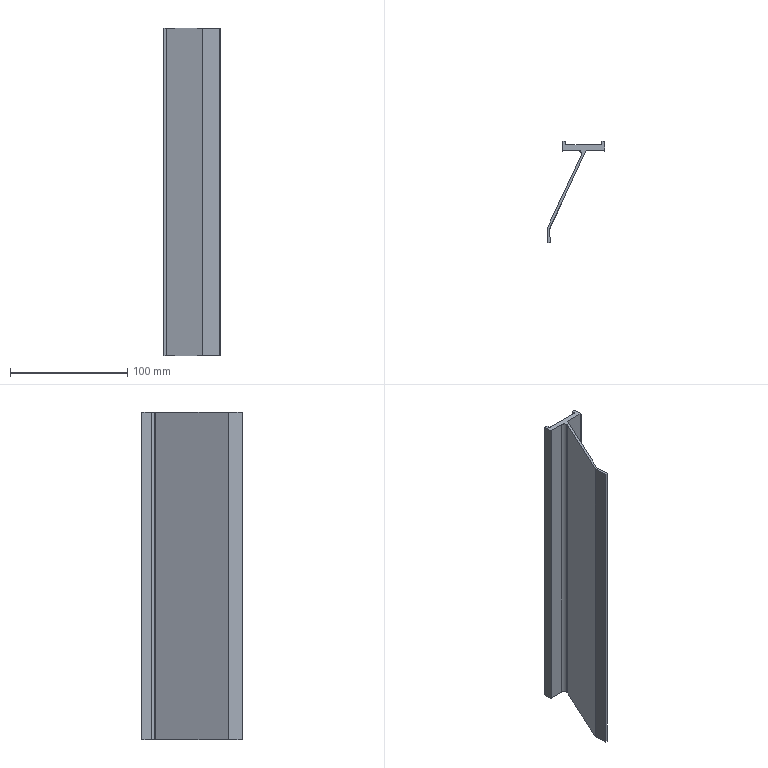Part | STEP file | Return squeegee | 1 solid | 22 faces | box 49.219 x 85.9 x 280 mm | volume 99161 mm3 | plane 18 | cylinder 4 | commonest cylinder face diameters 2 x2 6 x2
STEP:
#1=CARTESIAN_POINT('',(-4.916,-7.5,-280.));
#2=VERTEX_POINT('',#1);
#3=CARTESIAN_POINT('',(-1.916,-10.5,-280.));
#4=VERTEX_POINT('',#3);
#5=CARTESIAN_POINT('',(-4.916,-10.5,-280.));
#6=DIRECTION('',(0.,0.,-1.));
#7=DIRECTION('',(1.,0.,0.));
#8=AXIS2_PLACEMENT_3D('',#5,#6,#7);
#9=CIRCLE('',#8,3.);
#10=EDGE_CURVE('',#2,#4,#9,.T.);
#11=ORIENTED_EDGE('',*,*,#10,.T.);
#12=CARTESIAN_POINT('',(-1.916,-10.5,0.));
#13=VERTEX_POINT('',#12);
#14=CARTESIAN_POINT('',(-1.916,-10.5,-280.));
#15=DIRECTION('',(0.,0.,1.));
#16=VECTOR('',#15,1000.);
#17=LINE('',#14,#16);
#18=EDGE_CURVE('',#4,#13,#17,.T.);
#19=ORIENTED_EDGE('',*,*,#18,.T.);
#20=CARTESIAN_POINT('',(-4.916,-7.5,0.));
#21=VERTEX_POINT('',#20);
#22=CARTESIAN_POINT('',(-4.916,-10.5,0.));
#23=DIRECTION('',(0.,0.,-1.));
#24=DIRECTION('',(1.,0.,0.));
#25=AXIS2_PLACEMENT_3D('',#22,#23,#24);
#26=CIRCLE('',#25,3.);
#27=EDGE_CURVE('',#21,#13,#26,.T.);
#28=ORIENTED_EDGE('',*,*,#27,.F.);
#29=CARTESIAN_POINT('',(-4.916,-7.5,-280.));
#30=DIRECTION('',(0.,0.,1.));
#31=VECTOR('',#30,1000.);
#32=LINE('',#29,#31);
#33=EDGE_CURVE('',#2,#21,#32,.T.);
#34=ORIENTED_EDGE('',*,*,#33,.F.);
#35=EDGE_LOOP('',(#11,#19,#28,#34));
#36=FACE_OUTER_BOUND('',#35,.T.);
#37=CARTESIAN_POINT('',(-4.916,-10.5,-280.));
#38=DIRECTION('',(0.,0.,1.));
#39=DIRECTION('',(1.,0.,0.));
#40=AXIS2_PLACEMENT_3D('',#37,#38,#39);
#41=CYLINDRICAL_SURFACE('',#40,3.);
#42=ADVANCED_FACE('',(#36),#41,.F.);
#43=CARTESIAN_POINT('',(-15.5,0.,0.));
#44=VERTEX_POINT('',#43);
#45=CARTESIAN_POINT('',(-18.,0.,0.));
#46=VERTEX_POINT('',#45);
#47=CARTESIAN_POINT('',(-18.,0.,0.));
#48=DIRECTION('',(-1.,0.,0.));
#49=VECTOR('',#48,1000.);
#50=LINE('',#47,#49);
#51=EDGE_CURVE('',#44,#46,#50,.T.);
#52=ORIENTED_EDGE('',*,*,#51,.F.);
#53=CARTESIAN_POINT('',(-15.5,0.,-280.));
#54=VERTEX_POINT('',#53);
#55=CARTESIAN_POINT('',(-15.5,0.,-280.));
#56=DIRECTION('',(0.,0.,1.));
#57=VECTOR('',#56,1000.);
#58=LINE('',#55,#57);
#59=EDGE_CURVE('',#54,#44,#58,.T.);
#60=ORIENTED_EDGE('',*,*,#59,.F.);
#61=CARTESIAN_POINT('',(-18.,0.,-280.));
#62=VERTEX_POINT('',#61);
#63=CARTESIAN_POINT('',(-18.,0.,-280.));
#64=DIRECTION('',(-1.,0.,0.));
#65=VECTOR('',#64,1000.);
#66=LINE('',#63,#65);
#67=EDGE_CURVE('',#54,#62,#66,.T.);
#68=ORIENTED_EDGE('',*,*,#67,.T.);
#69=CARTESIAN_POINT('',(-18.,0.,-280.));
#70=DIRECTION('',(0.,0.,1.));
#71=VECTOR('',#70,1000.);
#72=LINE('',#69,#71);
#73=EDGE_CURVE('',#62,#46,#72,.T.);
#74=ORIENTED_EDGE('',*,*,#73,.T.);
#75=EDGE_LOOP('',(#52,#60,#68,#74));
#76=FACE_OUTER_BOUND('',#75,.T.);
#77=CARTESIAN_POINT('',(-18.,0.,-280.));
#78=DIRECTION('',(0.,1.,0.));
#79=DIRECTION('',(-1.,0.,0.));
#80=AXIS2_PLACEMENT_3D('',#77,#78,#79);
#81=PLANE('',#80);
#82=ADVANCED_FACE('',(#76),#81,.T.);
#83=CARTESIAN_POINT('',(-15.5,-2.,0.));
#84=VERTEX_POINT('',#83);
#85=CARTESIAN_POINT('',(-15.5,0.,0.));
#86=DIRECTION('',(0.,1.,0.));
#87=VECTOR('',#86,1000.);
#88=LINE('',#85,#87);
#89=EDGE_CURVE('',#84,#44,#88,.T.);
#90=ORIENTED_EDGE('',*,*,#89,.F.);
#91=CARTESIAN_POINT('',(-15.5,-2.,-280.));
#92=VERTEX_POINT('',#91);
#93=CARTESIAN_POINT('',(-15.5,-2.,-280.));
#94=DIRECTION('',(0.,0.,1.));
#95=VECTOR('',#94,1000.);
#96=LINE('',#93,#95);
#97=EDGE_CURVE('',#92,#84,#96,.T.);
#98=ORIENTED_EDGE('',*,*,#97,.F.);
#99=CARTESIAN_POINT('',(-15.5,0.,-280.));
#100=DIRECTION('',(0.,1.,0.));
#101=VECTOR('',#100,1000.);
#102=LINE('',#99,#101);
#103=EDGE_CURVE('',#92,#54,#102,.T.);
#104=ORIENTED_EDGE('',*,*,#103,.T.);
#105=ORIENTED_EDGE('',*,*,#59,.T.);
#106=EDGE_LOOP('',(#90,#98,#104,#105));
#107=FACE_OUTER_BOUND('',#106,.T.);
#108=CARTESIAN_POINT('',(-15.5,0.,-280.));
#109=DIRECTION('',(1.,0.,0.));
#110=DIRECTION('',(0.,1.,0.));
#111=AXIS2_PLACEMENT_3D('',#108,#109,#110);
#112=PLANE('',#111);
#113=ADVANCED_FACE('',(#107),#112,.T.);
#114=CARTESIAN_POINT('',(-14.5,-3.,0.));
#115=VERTEX_POINT('',#114);
#116=CARTESIAN_POINT('',(-14.5,-2.,0.));
#117=DIRECTION('',(0.,0.,-1.));
#118=DIRECTION('',(-1.,0.,0.));
#119=AXIS2_PLACEMENT_3D('',#116,#117,#118);
#120=CIRCLE('',#119,1.);
#121=EDGE_CURVE('',#115,#84,#120,.T.);
#122=ORIENTED_EDGE('',*,*,#121,.F.);
#123=CARTESIAN_POINT('',(-14.5,-3.,-280.));
#124=VERTEX_POINT('',#123);
#125=CARTESIAN_POINT('',(-14.5,-3.,-280.));
#126=DIRECTION('',(0.,0.,1.));
#127=VECTOR('',#126,1000.);
#128=LINE('',#125,#127);
#129=EDGE_CURVE('',#124,#115,#128,.T.);
#130=ORIENTED_EDGE('',*,*,#129,.F.);
#131=CARTESIAN_POINT('',(-14.5,-2.,-280.));
#132=DIRECTION('',(0.,0.,-1.));
#133=DIRECTION('',(-1.,0.,0.));
#134=AXIS2_PLACEMENT_3D('',#131,#132,#133);
#135=CIRCLE('',#134,1.);
#136=EDGE_CURVE('',#124,#92,#135,.T.);
#137=ORIENTED_EDGE('',*,*,#136,.T.);
#138=ORIENTED_EDGE('',*,*,#97,.T.);
#139=EDGE_LOOP('',(#122,#130,#137,#138));
#140=FACE_OUTER_BOUND('',#139,.T.);
#141=CARTESIAN_POINT('',(-14.5,-2.,-280.));
#142=DIRECTION('',(0.,0.,1.));
#143=DIRECTION('',(1.,0.,0.));
#144=AXIS2_PLACEMENT_3D('',#141,#142,#143);
#145=CYLINDRICAL_SURFACE('',#144,1.);
#146=ADVANCED_FACE('',(#140),#145,.F.);
#147=CARTESIAN_POINT('',(14.5,-3.,0.));
#148=VERTEX_POINT('',#147);
#149=CARTESIAN_POINT('',(-14.5,-3.,0.));
#150=DIRECTION('',(-1.,0.,0.));
#151=VECTOR('',#150,1000.);
#152=LINE('',#149,#151);
#153=EDGE_CURVE('',#148,#115,#152,.T.);
#154=ORIENTED_EDGE('',*,*,#153,.F.);
#155=CARTESIAN_POINT('',(14.5,-3.,-280.));
#156=VERTEX_POINT('',#155);
#157=CARTESIAN_POINT('',(14.5,-3.,-280.));
#158=DIRECTION('',(0.,0.,1.));
#159=VECTOR('',#158,1000.);
#160=LINE('',#157,#159);
#161=EDGE_CURVE('',#156,#148,#160,.T.);
#162=ORIENTED_EDGE('',*,*,#161,.F.);
#163=CARTESIAN_POINT('',(-14.5,-3.,-280.));
#164=DIRECTION('',(-1.,0.,0.));
#165=VECTOR('',#164,1000.);
#166=LINE('',#163,#165);
#167=EDGE_CURVE('',#156,#124,#166,.T.);
#168=ORIENTED_EDGE('',*,*,#167,.T.);
#169=ORIENTED_EDGE('',*,*,#129,.T.);
#170=EDGE_LOOP('',(#154,#162,#168,#169));
#171=FACE_OUTER_BOUND('',#170,.T.);
#172=CARTESIAN_POINT('',(-14.5,-3.,-280.));
#173=DIRECTION('',(0.,1.,0.));
#174=DIRECTION('',(-1.,0.,0.));
#175=AXIS2_PLACEMENT_3D('',#172,#173,#174);
#176=PLANE('',#175);
#177=ADVANCED_FACE('',(#171),#176,.T.);
#178=CARTESIAN_POINT('',(15.5,-2.,0.));
#179=VERTEX_POINT('',#178);
#180=CARTESIAN_POINT('',(14.5,-2.,0.));
#181=DIRECTION('',(0.,0.,-1.));
#182=DIRECTION('',(-1.,0.,0.));
#183=AXIS2_PLACEMENT_3D('',#180,#181,#182);
#184=CIRCLE('',#183,1.);
#185=EDGE_CURVE('',#179,#148,#184,.T.);
#186=ORIENTED_EDGE('',*,*,#185,.F.);
#187=CARTESIAN_POINT('',(15.5,-2.,-280.));
#188=VERTEX_POINT('',#187);
#189=CARTESIAN_POINT('',(15.5,-2.,-280.));
#190=DIRECTION('',(0.,0.,1.));
#191=VECTOR('',#190,1000.);
#192=LINE('',#189,#191);
#193=EDGE_CURVE('',#188,#179,#192,.T.);
#194=ORIENTED_EDGE('',*,*,#193,.F.);
#195=CARTESIAN_POINT('',(14.5,-2.,-280.));
#196=DIRECTION('',(0.,0.,-1.));
#197=DIRECTION('',(-1.,0.,0.));
#198=AXIS2_PLACEMENT_3D('',#195,#196,#197);
#199=CIRCLE('',#198,1.);
#200=EDGE_CURVE('',#188,#156,#199,.T.);
#201=ORIENTED_EDGE('',*,*,#200,.T.);
#202=ORIENTED_EDGE('',*,*,#161,.T.);
#203=EDGE_LOOP('',(#186,#194,#201,#202));
#204=FACE_OUTER_BOUND('',#203,.T.);
#205=CARTESIAN_POINT('',(14.5,-2.,-280.));
#206=DIRECTION('',(0.,0.,1.));
#207=DIRECTION('',(1.,0.,0.));
#208=AXIS2_PLACEMENT_3D('',#205,#206,#207);
#209=CYLINDRICAL_SURFACE('',#208,1.);
#210=ADVANCED_FACE('',(#204),#209,.F.);
#211=CARTESIAN_POINT('',(15.5,0.,0.));
#212=VERTEX_POINT('',#211);
#213=CARTESIAN_POINT('',(15.5,-2.,0.));
#214=DIRECTION('',(0.,-1.,0.));
#215=VECTOR('',#214,1000.);
#216=LINE('',#213,#215);
#217=EDGE_CURVE('',#212,#179,#216,.T.);
#218=ORIENTED_EDGE('',*,*,#217,.F.);
#219=CARTESIAN_POINT('',(15.5,0.,-280.));
#220=VERTEX_POINT('',#219);
#221=CARTESIAN_POINT('',(15.5,0.,-280.));
#222=DIRECTION('',(0.,0.,1.));
#223=VECTOR('',#222,1000.);
#224=LINE('',#221,#223);
#225=EDGE_CURVE('',#220,#212,#224,.T.);
#226=ORIENTED_EDGE('',*,*,#225,.F.);
#227=CARTESIAN_POINT('',(15.5,-2.,-280.));
#228=DIRECTION('',(0.,-1.,0.));
#229=VECTOR('',#228,1000.);
#230=LINE('',#227,#229);
#231=EDGE_CURVE('',#220,#188,#230,.T.);
#232=ORIENTED_EDGE('',*,*,#231,.T.);
#233=ORIENTED_EDGE('',*,*,#193,.T.);
#234=EDGE_LOOP('',(#218,#226,#232,#233));
#235=FACE_OUTER_BOUND('',#234,.T.);
#236=CARTESIAN_POINT('',(15.5,-2.,-280.));
#237=DIRECTION('',(-1.,0.,0.));
#238=DIRECTION('',(0.,-1.,0.));
#239=AXIS2_PLACEMENT_3D('',#236,#237,#238);
#240=PLANE('',#239);
#241=ADVANCED_FACE('',(#235),#240,.T.);
#242=CARTESIAN_POINT('',(18.,0.,0.));
#243=VERTEX_POINT('',#242);
#244=CARTESIAN_POINT('',(15.5,0.,0.));
#245=DIRECTION('',(-1.,0.,0.));
#246=VECTOR('',#245,1000.);
#247=LINE('',#244,#246);
#248=EDGE_CURVE('',#243,#212,#247,.T.);
#249=ORIENTED_EDGE('',*,*,#248,.F.);
#250=CARTESIAN_POINT('',(18.,0.,-280.));
#251=VERTEX_POINT('',#250);
#252=CARTESIAN_POINT('',(18.,0.,-280.));
#253=DIRECTION('',(0.,0.,1.));
#254=VECTOR('',#253,1000.);
#255=LINE('',#252,#254);
#256=EDGE_CURVE('',#251,#243,#255,.T.);
#257=ORIENTED_EDGE('',*,*,#256,.F.);
#258=CARTESIAN_POINT('',(15.5,0.,-280.));
#259=DIRECTION('',(-1.,0.,0.));
#260=VECTOR('',#259,1000.);
#261=LINE('',#258,#260);
#262=EDGE_CURVE('',#251,#220,#261,.T.);
#263=ORIENTED_EDGE('',*,*,#262,.T.);
#264=ORIENTED_EDGE('',*,*,#225,.T.);
#265=EDGE_LOOP('',(#249,#257,#263,#264));
#266=FACE_OUTER_BOUND('',#265,.T.);
#267=CARTESIAN_POINT('',(15.5,0.,-280.));
#268=DIRECTION('',(0.,1.,0.));
#269=DIRECTION('',(-1.,0.,0.));
#270=AXIS2_PLACEMENT_3D('',#267,#268,#269);
#271=PLANE('',#270);
#272=ADVANCED_FACE('',(#266),#271,.T.);
#273=CARTESIAN_POINT('',(18.,-8.5,0.));
#274=VERTEX_POINT('',#273);
#275=CARTESIAN_POINT('',(18.,0.,0.));
#276=DIRECTION('',(0.,1.,0.));
#277=VECTOR('',#276,1000.);
#278=LINE('',#275,#277);
#279=EDGE_CURVE('',#274,#243,#278,.T.);
#280=ORIENTED_EDGE('',*,*,#279,.F.);
#281=CARTESIAN_POINT('',(18.,-8.5,-280.));
#282=VERTEX_POINT('',#281);
#283=CARTESIAN_POINT('',(18.,-8.5,-280.));
#284=DIRECTION('',(0.,0.,1.));
#285=VECTOR('',#284,1000.);
#286=LINE('',#283,#285);
#287=EDGE_CURVE('',#282,#274,#286,.T.);
#288=ORIENTED_EDGE('',*,*,#287,.F.);
#289=CARTESIAN_POINT('',(18.,0.,-280.));
#290=DIRECTION('',(0.,1.,0.));
#291=VECTOR('',#290,1000.);
#292=LINE('',#289,#291);
#293=EDGE_CURVE('',#282,#251,#292,.T.);
#294=ORIENTED_EDGE('',*,*,#293,.T.);
#295=ORIENTED_EDGE('',*,*,#256,.T.);
#296=EDGE_LOOP('',(#280,#288,#294,#295));
#297=FACE_OUTER_BOUND('',#296,.T.);
#298=CARTESIAN_POINT('',(18.,0.,-280.));
#299=DIRECTION('',(1.,0.,0.));
#300=DIRECTION('',(0.,1.,0.));
#301=AXIS2_PLACEMENT_3D('',#298,#299,#300);
#302=PLANE('',#301);
#303=ADVANCED_FACE('',(#297),#302,.T.);
#304=CARTESIAN_POINT('',(17.,-7.5,0.));
#305=VERTEX_POINT('',#304);
#306=CARTESIAN_POINT('',(17.,-7.5,0.));
#307=DIRECTION('',(0.7071,-0.7071,0.));
#308=VECTOR('',#307,1000.);
#309=LINE('',#306,#308);
#310=EDGE_CURVE('',#305,#274,#309,.T.);
#311=ORIENTED_EDGE('',*,*,#310,.F.);
#312=CARTESIAN_POINT('',(17.,-7.5,-280.));
#313=VERTEX_POINT('',#312);
#314=CARTESIAN_POINT('',(17.,-7.5,-280.));
#315=DIRECTION('',(0.,0.,1.));
#316=VECTOR('',#315,1000.);
#317=LINE('',#314,#316);
#318=EDGE_CURVE('',#313,#305,#317,.T.);
#319=ORIENTED_EDGE('',*,*,#318,.F.);
#320=CARTESIAN_POINT('',(17.,-7.5,-280.));
#321=DIRECTION('',(0.7071,-0.7071,0.));
#322=VECTOR('',#321,1000.);
#323=LINE('',#320,#322);
#324=EDGE_CURVE('',#313,#282,#323,.T.);
#325=ORIENTED_EDGE('',*,*,#324,.T.);
#326=ORIENTED_EDGE('',*,*,#287,.T.);
#327=EDGE_LOOP('',(#311,#319,#325,#326));
#328=FACE_OUTER_BOUND('',#327,.T.);
#329=CARTESIAN_POINT('',(17.,-7.5,-280.));
#330=DIRECTION('',(-0.7071,-0.7071,0.));
#331=DIRECTION('',(0.7071,-0.7071,0.));
#332=AXIS2_PLACEMENT_3D('',#329,#330,#331);
#333=PLANE('',#332);
#334=ADVANCED_FACE('',(#328),#333,.T.);
#335=CARTESIAN_POINT('',(2.,-7.5,0.));
#336=VERTEX_POINT('',#335);
#337=CARTESIAN_POINT('',(2.,-7.5,0.));
#338=DIRECTION('',(1.,0.,0.));
#339=VECTOR('',#338,1000.);
#340=LINE('',#337,#339);
#341=EDGE_CURVE('',#336,#305,#340,.T.);
#342=ORIENTED_EDGE('',*,*,#341,.F.);
#343=CARTESIAN_POINT('',(2.,-7.5,-280.));
#344=VERTEX_POINT('',#343);
#345=CARTESIAN_POINT('',(2.,-7.5,-280.));
#346=DIRECTION('',(0.,0.,1.));
#347=VECTOR('',#346,1000.);
#348=LINE('',#345,#347);
#349=EDGE_CURVE('',#344,#336,#348,.T.);
#350=ORIENTED_EDGE('',*,*,#349,.F.);
#351=CARTESIAN_POINT('',(2.,-7.5,-280.));
#352=DIRECTION('',(1.,0.,0.));
#353=VECTOR('',#352,1000.);
#354=LINE('',#351,#353);
#355=EDGE_CURVE('',#344,#313,#354,.T.);
#356=ORIENTED_EDGE('',*,*,#355,.T.);
#357=ORIENTED_EDGE('',*,*,#318,.T.);
#358=EDGE_LOOP('',(#342,#350,#356,#357));
#359=FACE_OUTER_BOUND('',#358,.T.);
#360=CARTESIAN_POINT('',(2.,-7.5,-280.));
#361=DIRECTION('',(0.,-1.,0.));
#362=DIRECTION('',(1.,0.,0.));
#363=AXIS2_PLACEMENT_3D('',#360,#361,#362);
#364=PLANE('',#363);
#365=ADVANCED_FACE('',(#359),#364,.T.);
#366=CARTESIAN_POINT('',(-29.196,-74.4,0.));
#367=VERTEX_POINT('',#366);
#368=CARTESIAN_POINT('',(2.,-7.5,0.));
#369=DIRECTION('',(0.4226,0.9063,0.));
#370=VECTOR('',#369,1000.);
#371=LINE('',#368,#370);
#372=EDGE_CURVE('',#367,#336,#371,.T.);
#373=ORIENTED_EDGE('',*,*,#372,.F.);
#374=CARTESIAN_POINT('',(-29.196,-74.4,-280.));
#375=VERTEX_POINT('',#374);
#376=CARTESIAN_POINT('',(-29.196,-74.4,-280.));
#377=DIRECTION('',(0.,0.,1.));
#378=VECTOR('',#377,1000.);
#379=LINE('',#376,#378);
#380=EDGE_CURVE('',#375,#367,#379,.T.);
#381=ORIENTED_EDGE('',*,*,#380,.F.);
#382=CARTESIAN_POINT('',(2.,-7.5,-280.));
#383=DIRECTION('',(0.4226,0.9063,0.));
#384=VECTOR('',#383,1000.);
#385=LINE('',#382,#384);
#386=EDGE_CURVE('',#375,#344,#385,.T.);
#387=ORIENTED_EDGE('',*,*,#386,.T.);
#388=ORIENTED_EDGE('',*,*,#349,.T.);
#389=EDGE_LOOP('',(#373,#381,#387,#388));
#390=FACE_OUTER_BOUND('',#389,.T.);
#391=CARTESIAN_POINT('',(2.,-7.5,-280.));
#392=DIRECTION('',(0.9063,-0.4226,0.));
#393=DIRECTION('',(0.4226,0.9063,0.));
#394=AXIS2_PLACEMENT_3D('',#391,#392,#393);
#395=PLANE('',#394);
#396=ADVANCED_FACE('',(#390),#395,.T.);
#397=CARTESIAN_POINT('',(-28.593,-85.9,0.));
#398=VERTEX_POINT('',#397);
#399=CARTESIAN_POINT('',(-29.196,-74.4,0.));
#400=DIRECTION('',(-0.05234,0.9986,0.));
#401=VECTOR('',#400,1000.);
#402=LINE('',#399,#401);
#403=EDGE_CURVE('',#398,#367,#402,.T.);
#404=ORIENTED_EDGE('',*,*,#403,.F.);
#405=CARTESIAN_POINT('',(-28.593,-85.9,-280.));
#406=VERTEX_POINT('',#405);
#407=CARTESIAN_POINT('',(-28.593,-85.9,-280.));
#408=DIRECTION('',(0.,0.,1.));
#409=VECTOR('',#408,1000.);
#410=LINE('',#407,#409);
#411=EDGE_CURVE('',#406,#398,#410,.T.);
#412=ORIENTED_EDGE('',*,*,#411,.F.);
#413=CARTESIAN_POINT('',(-29.196,-74.4,-280.));
#414=DIRECTION('',(-0.05234,0.9986,0.));
#415=VECTOR('',#414,1000.);
#416=LINE('',#413,#415);
#417=EDGE_CURVE('',#406,#375,#416,.T.);
#418=ORIENTED_EDGE('',*,*,#417,.T.);
#419=ORIENTED_EDGE('',*,*,#380,.T.);
#420=EDGE_LOOP('',(#404,#412,#418,#419));
#421=FACE_OUTER_BOUND('',#420,.T.);
#422=CARTESIAN_POINT('',(-29.196,-74.4,-280.));
#423=DIRECTION('',(0.9986,0.05234,0.));
#424=DIRECTION('',(-0.05234,0.9986,0.));
#425=AXIS2_PLACEMENT_3D('',#422,#423,#424);
#426=PLANE('',#425);
#427=ADVANCED_FACE('',(#421),#426,.T.);
#428=CARTESIAN_POINT('',(-30.596,-85.9,0.));
#429=VERTEX_POINT('',#428);
#430=CARTESIAN_POINT('',(-28.593,-85.9,0.));
#431=DIRECTION('',(1.,0.,0.));
#432=VECTOR('',#431,1000.);
#433=LINE('',#430,#432);
#434=EDGE_CURVE('',#429,#398,#433,.T.);
#435=ORIENTED_EDGE('',*,*,#434,.F.);
#436=CARTESIAN_POINT('',(-30.596,-85.9,-280.));
#437=VERTEX_POINT('',#436);
#438=CARTESIAN_POINT('',(-30.596,-85.9,-280.));
#439=DIRECTION('',(0.,0.,1.));
#440=VECTOR('',#439,1000.);
#441=LINE('',#438,#440);
#442=EDGE_CURVE('',#437,#429,#441,.T.);
#443=ORIENTED_EDGE('',*,*,#442,.F.);
#444=CARTESIAN_POINT('',(-28.593,-85.9,-280.));
#445=DIRECTION('',(1.,0.,0.));
#446=VECTOR('',#445,1000.);
#447=LINE('',#444,#446);
#448=EDGE_CURVE('',#437,#406,#447,.T.);
#449=ORIENTED_EDGE('',*,*,#448,.T.);
#450=ORIENTED_EDGE('',*,*,#411,.T.);
#451=EDGE_LOOP('',(#435,#443,#449,#450));
#452=FACE_OUTER_BOUND('',#451,.T.);
#453=CARTESIAN_POINT('',(-28.593,-85.9,-280.));
#454=DIRECTION('',(0.,-1.,0.));
#455=DIRECTION('',(0.,0.,-1.));
#456=AXIS2_PLACEMENT_3D('',#453,#454,#455);
#457=PLANE('',#456);
#458=ADVANCED_FACE('',(#452),#457,.T.);
#459=CARTESIAN_POINT('',(-31.219,-74.007,0.));
#460=VERTEX_POINT('',#459);
#461=CARTESIAN_POINT('',(-30.596,-85.9,0.));
#462=DIRECTION('',(0.05234,-0.9986,0.));
#463=VECTOR('',#462,1000.);
#464=LINE('',#461,#463);
#465=EDGE_CURVE('',#460,#429,#464,.T.);
#466=ORIENTED_EDGE('',*,*,#465,.F.);
#467=CARTESIAN_POINT('',(-31.219,-74.007,-280.));
#468=VERTEX_POINT('',#467);
#469=CARTESIAN_POINT('',(-31.219,-74.007,-280.));
#470=DIRECTION('',(0.,0.,1.));
#471=VECTOR('',#470,1000.);
#472=LINE('',#469,#471);
#473=EDGE_CURVE('',#468,#460,#472,.T.);
#474=ORIENTED_EDGE('',*,*,#473,.F.);
#475=CARTESIAN_POINT('',(-30.596,-85.9,-280.));
#476=DIRECTION('',(0.05234,-0.9986,0.));
#477=VECTOR('',#476,1000.);
#478=LINE('',#475,#477);
#479=EDGE_CURVE('',#468,#437,#478,.T.);
#480=ORIENTED_EDGE('',*,*,#479,.T.);
#481=ORIENTED_EDGE('',*,*,#442,.T.);
#482=EDGE_LOOP('',(#466,#474,#480,#481));
#483=FACE_OUTER_BOUND('',#482,.T.);
#484=CARTESIAN_POINT('',(-30.596,-85.9,-280.));
#485=DIRECTION('',(-0.9986,-0.05234,0.));
#486=DIRECTION('',(0.05234,-0.9986,0.));
#487=AXIS2_PLACEMENT_3D('',#484,#485,#486);
#488=PLANE('',#487);
#489=ADVANCED_FACE('',(#483),#488,.T.);
#490=CARTESIAN_POINT('',(-2.197,-11.768,0.));
#491=VERTEX_POINT('',#490);
#492=CARTESIAN_POINT('',(-31.219,-74.007,0.));
#493=DIRECTION('',(-0.4226,-0.9063,0.));
#494=VECTOR('',#493,1000.);
#495=LINE('',#492,#494);
#496=EDGE_CURVE('',#491,#460,#495,.T.);
#497=ORIENTED_EDGE('',*,*,#496,.F.);
#498=CARTESIAN_POINT('',(-2.197,-11.768,-280.));
#499=VERTEX_POINT('',#498);
#500=CARTESIAN_POINT('',(-2.197,-11.768,-280.));
#501=DIRECTION('',(0.,0.,1.));
#502=VECTOR('',#501,1000.);
#503=LINE('',#500,#502);
#504=EDGE_CURVE('',#499,#491,#503,.T.);
#505=ORIENTED_EDGE('',*,*,#504,.F.);
#506=CARTESIAN_POINT('',(-31.219,-74.007,-280.));
#507=DIRECTION('',(-0.4226,-0.9063,0.));
#508=VECTOR('',#507,1000.);
#509=LINE('',#506,#508);
#510=EDGE_CURVE('',#499,#468,#509,.T.);
#511=ORIENTED_EDGE('',*,*,#510,.T.);
#512=ORIENTED_EDGE('',*,*,#473,.T.);
#513=EDGE_LOOP('',(#497,#505,#511,#512));
#514=FACE_OUTER_BOUND('',#513,.T.);
#515=CARTESIAN_POINT('',(-31.219,-74.007,-280.));
#516=DIRECTION('',(-0.9063,0.4226,0.));
#517=DIRECTION('',(-0.4226,-0.9063,0.));
#518=AXIS2_PLACEMENT_3D('',#515,#516,#517);
#519=PLANE('',#518);
#520=ADVANCED_FACE('',(#514),#519,.T.);
#521=ORIENTED_EDGE('',*,*,#18,.F.);
#522=CARTESIAN_POINT('',(-4.916,-10.5,-280.));
#523=DIRECTION('',(0.,0.,-1.));
#524=DIRECTION('',(1.,0.,0.));
#525=AXIS2_PLACEMENT_3D('',#522,#523,#524);
#526=CIRCLE('',#525,3.);
#527=EDGE_CURVE('',#4,#499,#526,.T.);
#528=ORIENTED_EDGE('',*,*,#527,.T.);
#529=ORIENTED_EDGE('',*,*,#504,.T.);
#530=CARTESIAN_POINT('',(-4.916,-10.5,0.));
#531=DIRECTION('',(0.,0.,-1.));
#532=DIRECTION('',(1.,0.,0.));
#533=AXIS2_PLACEMENT_3D('',#530,#531,#532);
#534=CIRCLE('',#533,3.);
#535=EDGE_CURVE('',#13,#491,#534,.T.);
#536=ORIENTED_EDGE('',*,*,#535,.F.);
#537=EDGE_LOOP('',(#521,#528,#529,#536));
#538=FACE_OUTER_BOUND('',#537,.T.);
#539=CARTESIAN_POINT('',(-4.916,-10.5,-280.));
#540=DIRECTION('',(0.,0.,1.));
#541=DIRECTION('',(1.,0.,0.));
#542=AXIS2_PLACEMENT_3D('',#539,#540,#541);
#543=CYLINDRICAL_SURFACE('',#542,3.);
#544=ADVANCED_FACE('',(#538),#543,.F.);
#545=CARTESIAN_POINT('',(-17.,-7.5,0.));
#546=VERTEX_POINT('',#545);
#547=CARTESIAN_POINT('',(-4.916,-7.5,0.));
#548=DIRECTION('',(1.,0.,0.));
#549=VECTOR('',#548,1000.);
#550=LINE('',#547,#549);
#551=EDGE_CURVE('',#546,#21,#550,.T.);
#552=ORIENTED_EDGE('',*,*,#551,.F.);
#553=CARTESIAN_POINT('',(-17.,-7.5,-280.));
#554=VERTEX_POINT('',#553);
#555=CARTESIAN_POINT('',(-17.,-7.5,-280.));
#556=DIRECTION('',(0.,0.,1.));
#557=VECTOR('',#556,1000.);
#558=LINE('',#555,#557);
#559=EDGE_CURVE('',#554,#546,#558,.T.);
#560=ORIENTED_EDGE('',*,*,#559,.F.);
#561=CARTESIAN_POINT('',(-4.916,-7.5,-280.));
#562=DIRECTION('',(1.,0.,0.));
#563=VECTOR('',#562,1000.);
#564=LINE('',#561,#563);
#565=EDGE_CURVE('',#554,#2,#564,.T.);
#566=ORIENTED_EDGE('',*,*,#565,.T.);
#567=ORIENTED_EDGE('',*,*,#33,.T.);
#568=EDGE_LOOP('',(#552,#560,#566,#567));
#569=FACE_OUTER_BOUND('',#568,.T.);
#570=CARTESIAN_POINT('',(-4.916,-7.5,-280.));
#571=DIRECTION('',(0.,-1.,0.));
#572=DIRECTION('',(1.,0.,0.));
#573=AXIS2_PLACEMENT_3D('',#570,#571,#572);
#574=PLANE('',#573);
#575=ADVANCED_FACE('',(#569),#574,.T.);
#576=CARTESIAN_POINT('',(-18.,-8.5,0.));
#577=VERTEX_POINT('',#576);
#578=CARTESIAN_POINT('',(-17.,-7.5,0.));
#579=DIRECTION('',(0.7071,0.7071,0.));
#580=VECTOR('',#579,1000.);
#581=LINE('',#578,#580);
#582=EDGE_CURVE('',#577,#546,#581,.T.);
#583=ORIENTED_EDGE('',*,*,#582,.F.);
#584=CARTESIAN_POINT('',(-18.,-8.5,-280.));
#585=VERTEX_POINT('',#584);
#586=CARTESIAN_POINT('',(-18.,-8.5,-280.));
#587=DIRECTION('',(0.,0.,1.));
#588=VECTOR('',#587,1000.);
#589=LINE('',#586,#588);
#590=EDGE_CURVE('',#585,#577,#589,.T.);
#591=ORIENTED_EDGE('',*,*,#590,.F.);
#592=CARTESIAN_POINT('',(-17.,-7.5,-280.));
#593=DIRECTION('',(0.7071,0.7071,0.));
#594=VECTOR('',#593,1000.);
#595=LINE('',#592,#594);
#596=EDGE_CURVE('',#585,#554,#595,.T.);
#597=ORIENTED_EDGE('',*,*,#596,.T.);
#598=ORIENTED_EDGE('',*,*,#559,.T.);
#599=EDGE_LOOP('',(#583,#591,#597,#598));
#600=FACE_OUTER_BOUND('',#599,.T.);
#601=CARTESIAN_POINT('',(-17.,-7.5,-280.));
#602=DIRECTION('',(0.7071,-0.7071,0.));
#603=DIRECTION('',(0.7071,0.7071,0.));
#604=AXIS2_PLACEMENT_3D('',#601,#602,#603);
#605=PLANE('',#604);
#606=ADVANCED_FACE('',(#600),#605,.T.);
#607=CARTESIAN_POINT('',(-18.,-8.5,0.));
#608=DIRECTION('',(0.,-1.,0.));
#609=VECTOR('',#608,1000.);
#610=LINE('',#607,#609);
#611=EDGE_CURVE('',#46,#577,#610,.T.);
#612=ORIENTED_EDGE('',*,*,#611,.F.);
#613=ORIENTED_EDGE('',*,*,#73,.F.);
#614=CARTESIAN_POINT('',(-18.,-8.5,-280.));
#615=DIRECTION('',(0.,-1.,0.));
#616=VECTOR('',#615,1000.);
#617=LINE('',#614,#616);
#618=EDGE_CURVE('',#62,#585,#617,.T.);
#619=ORIENTED_EDGE('',*,*,#618,.T.);
#620=ORIENTED_EDGE('',*,*,#590,.T.);
#621=EDGE_LOOP('',(#612,#613,#619,#620));
#622=FACE_OUTER_BOUND('',#621,.T.);
#623=CARTESIAN_POINT('',(-18.,-8.5,-280.));
#624=DIRECTION('',(-1.,0.,0.));
#625=DIRECTION('',(0.,-1.,0.));
#626=AXIS2_PLACEMENT_3D('',#623,#624,#625);
#627=PLANE('',#626);
#628=ADVANCED_FACE('',(#622),#627,.T.);
#629=ORIENTED_EDGE('',*,*,#67,.F.);
#630=ORIENTED_EDGE('',*,*,#103,.F.);
#631=ORIENTED_EDGE('',*,*,#136,.F.);
#632=ORIENTED_EDGE('',*,*,#167,.F.);
#633=ORIENTED_EDGE('',*,*,#200,.F.);
#634=ORIENTED_EDGE('',*,*,#231,.F.);
#635=ORIENTED_EDGE('',*,*,#262,.F.);
#636=ORIENTED_EDGE('',*,*,#293,.F.);
#637=ORIENTED_EDGE('',*,*,#324,.F.);
#638=ORIENTED_EDGE('',*,*,#355,.F.);
#639=ORIENTED_EDGE('',*,*,#386,.F.);
#640=ORIENTED_EDGE('',*,*,#417,.F.);
#641=ORIENTED_EDGE('',*,*,#448,.F.);
#642=ORIENTED_EDGE('',*,*,#479,.F.);
#643=ORIENTED_EDGE('',*,*,#510,.F.);
#644=ORIENTED_EDGE('',*,*,#527,.F.);
#645=ORIENTED_EDGE('',*,*,#10,.F.);
#646=ORIENTED_EDGE('',*,*,#565,.F.);
#647=ORIENTED_EDGE('',*,*,#596,.F.);
#648=ORIENTED_EDGE('',*,*,#618,.F.);
#649=EDGE_LOOP('',(#629,#630,#631,#632,#633,#634,#635,#636,#637,#638,#639,#640,#641,#642,#643,#644,#645,#646,#647,#648));
#650=FACE_OUTER_BOUND('',#649,.T.);
#651=CARTESIAN_POINT('',(-14.5,-2.,-280.));
#652=DIRECTION('',(0.,0.,-1.));
#653=DIRECTION('',(-1.,0.,0.));
#654=AXIS2_PLACEMENT_3D('',#651,#652,#653);
#655=PLANE('',#654);
#656=ADVANCED_FACE('',(#650),#655,.T.);
#657=ORIENTED_EDGE('',*,*,#51,.T.);
#658=ORIENTED_EDGE('',*,*,#611,.T.);
#659=ORIENTED_EDGE('',*,*,#582,.T.);
#660=ORIENTED_EDGE('',*,*,#551,.T.);
#661=ORIENTED_EDGE('',*,*,#27,.T.);
#662=ORIENTED_EDGE('',*,*,#535,.T.);
#663=ORIENTED_EDGE('',*,*,#496,.T.);
#664=ORIENTED_EDGE('',*,*,#465,.T.);
#665=ORIENTED_EDGE('',*,*,#434,.T.);
#666=ORIENTED_EDGE('',*,*,#403,.T.);
#667=ORIENTED_EDGE('',*,*,#372,.T.);
#668=ORIENTED_EDGE('',*,*,#341,.T.);
#669=ORIENTED_EDGE('',*,*,#310,.T.);
#670=ORIENTED_EDGE('',*,*,#279,.T.);
#671=ORIENTED_EDGE('',*,*,#248,.T.);
#672=ORIENTED_EDGE('',*,*,#217,.T.);
#673=ORIENTED_EDGE('',*,*,#185,.T.);
#674=ORIENTED_EDGE('',*,*,#153,.T.);
#675=ORIENTED_EDGE('',*,*,#121,.T.);
#676=ORIENTED_EDGE('',*,*,#89,.T.);
#677=EDGE_LOOP('',(#657,#658,#659,#660,#661,#662,#663,#664,#665,#666,#667,#668,#669,#670,#671,#672,#673,#674,#675,#676));
#678=FACE_OUTER_BOUND('',#677,.T.);
#679=CARTESIAN_POINT('',(-14.5,-2.,0.));
#680=DIRECTION('',(0.,0.,-1.));
#681=DIRECTION('',(-1.,0.,0.));
#682=AXIS2_PLACEMENT_3D('',#679,#680,#681);
#683=PLANE('',#682);
#684=ADVANCED_FACE('',(#678),#683,.F.);
#685=CLOSED_SHELL('',(#42,#82,#113,#146,#177,#210,#241,#272,#303,#334,#365,#396,#427,#458,#489,#520,#544,#575,#606,#628,#656,#684));
#686=MANIFOLD_SOLID_BREP('',#685);
#687=CARTESIAN_POINT('',(0.,0.,0.));
#688=DIRECTION('',(0.,0.,1.));
#689=DIRECTION('',(1.,0.,0.));
#690=AXIS2_PLACEMENT_3D('',#687,#688,#689);
#691=(LENGTH_UNIT()NAMED_UNIT(*)SI_UNIT(.MILLI.,.METRE.));
#692=UNCERTAINTY_MEASURE_WITH_UNIT(LENGTH_MEASURE(0.00001),#691,'','');
#693=(NAMED_UNIT(*)PLANE_ANGLE_UNIT()SI_UNIT($,.RADIAN.));
#694=(NAMED_UNIT(*)SI_UNIT($,.STERADIAN.)SOLID_ANGLE_UNIT());
#695=(GEOMETRIC_REPRESENTATION_CONTEXT(3)GLOBAL_UNCERTAINTY_ASSIGNED_CONTEXT((#692))GLOBAL_UNIT_ASSIGNED_CONTEXT((#691,#693,#694))REPRESENTATION_CONTEXT('',''));
#696=ADVANCED_BREP_SHAPE_REPRESENTATION('',(#686,#690),#695);